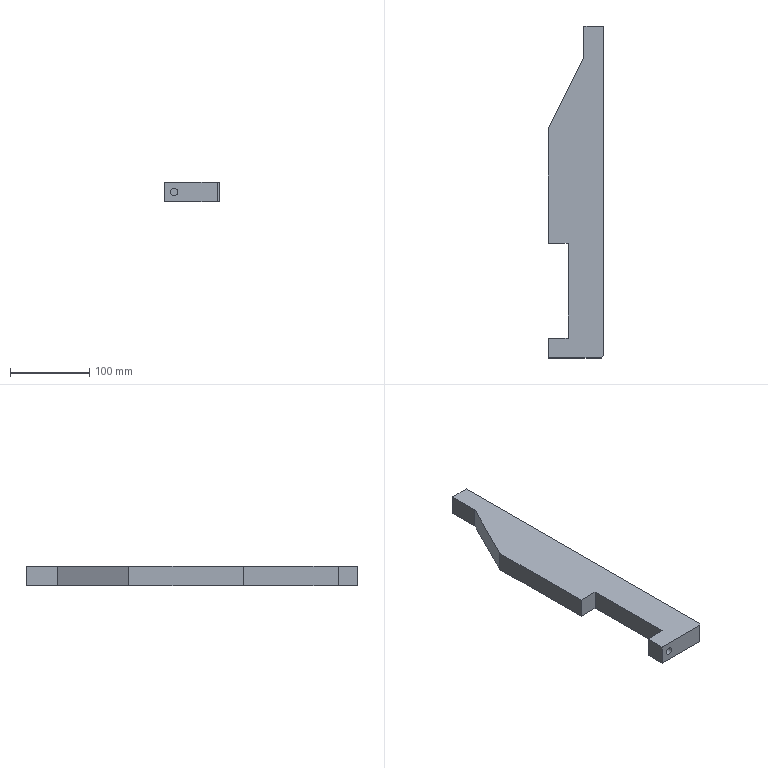Part | NX | 1 solid | 22 faces | box 70 x 420 x 25 mm | volume 559704 mm3 | plane 13 | cylinder 5 | cone 4 | commonest cylinder face diameters 6.8 x4 9 x1
STEP:
#1=CARTESIAN_POINT('',(67.,0.,12.5));
#2=VERTEX_POINT('',#1);
#3=CARTESIAN_POINT('',(70.,3.,12.5));
#4=VERTEX_POINT('',#3);
#5=CARTESIAN_POINT('',(33.5,-33.5,12.5));
#6=DIRECTION('',(0.7071,0.7071,0.));
#7=VECTOR('',#6,1000.);
#8=LINE('',#5,#7);
#9=EDGE_CURVE('',#2,#4,#8,.T.);
#10=ORIENTED_EDGE('',*,*,#9,.F.);
#11=CARTESIAN_POINT('',(67.,0.,-12.5));
#12=VERTEX_POINT('',#11);
#13=CARTESIAN_POINT('',(67.,0.,12.5));
#14=DIRECTION('',(0.,0.,1.));
#15=VECTOR('',#14,1000.);
#16=LINE('',#13,#15);
#17=EDGE_CURVE('',#12,#2,#16,.T.);
#18=ORIENTED_EDGE('',*,*,#17,.F.);
#19=CARTESIAN_POINT('',(70.,3.,-12.5));
#20=VERTEX_POINT('',#19);
#21=CARTESIAN_POINT('',(70.,3.,-12.5));
#22=DIRECTION('',(-0.7071,-0.7071,0.));
#23=VECTOR('',#22,1000.);
#24=LINE('',#21,#23);
#25=EDGE_CURVE('',#20,#12,#24,.T.);
#26=ORIENTED_EDGE('',*,*,#25,.F.);
#27=CARTESIAN_POINT('',(70.,3.,12.5));
#28=DIRECTION('',(0.,0.,-1.));
#29=VECTOR('',#28,1000.);
#30=LINE('',#27,#29);
#31=EDGE_CURVE('',#4,#20,#30,.T.);
#32=ORIENTED_EDGE('',*,*,#31,.F.);
#33=EDGE_LOOP('',(#10,#18,#26,#32));
#34=FACE_BOUND('',#33,.T.);
#35=CARTESIAN_POINT('',(70.,3.,12.5));
#36=DIRECTION('',(-0.7071,0.7071,0.));
#37=DIRECTION('',(0.,0.,-1.));
#38=AXIS2_PLACEMENT_3D('',#35,#36,#37);
#39=PLANE('',#38);
#40=ADVANCED_FACE('',(#34),#39,.F.);
#41=CARTESIAN_POINT('',(0.,290.,12.5));
#42=VERTEX_POINT('',#41);
#43=CARTESIAN_POINT('',(45.,380.,12.5));
#44=VERTEX_POINT('',#43);
#45=CARTESIAN_POINT('',(45.,380.,12.5));
#46=DIRECTION('',(0.4472,0.8944,0.));
#47=VECTOR('',#46,1000.);
#48=LINE('',#45,#47);
#49=EDGE_CURVE('',#42,#44,#48,.T.);
#50=ORIENTED_EDGE('',*,*,#49,.T.);
#51=CARTESIAN_POINT('',(45.,380.,-12.5));
#52=VERTEX_POINT('',#51);
#53=CARTESIAN_POINT('',(45.,380.,-12.5));
#54=DIRECTION('',(0.,0.,1.));
#55=VECTOR('',#54,1000.);
#56=LINE('',#53,#55);
#57=EDGE_CURVE('',#52,#44,#56,.T.);
#58=ORIENTED_EDGE('',*,*,#57,.F.);
#59=CARTESIAN_POINT('',(0.,290.,-12.5));
#60=VERTEX_POINT('',#59);
#61=CARTESIAN_POINT('',(45.,380.,-12.5));
#62=DIRECTION('',(0.4472,0.8944,0.));
#63=VECTOR('',#62,1000.);
#64=LINE('',#61,#63);
#65=EDGE_CURVE('',#60,#52,#64,.T.);
#66=ORIENTED_EDGE('',*,*,#65,.F.);
#67=CARTESIAN_POINT('',(0.,290.,-12.5));
#68=DIRECTION('',(0.,0.,1.));
#69=VECTOR('',#68,1000.);
#70=LINE('',#67,#69);
#71=EDGE_CURVE('',#60,#42,#70,.T.);
#72=ORIENTED_EDGE('',*,*,#71,.T.);
#73=EDGE_LOOP('',(#50,#58,#66,#72));
#74=FACE_BOUND('',#73,.T.);
#75=CARTESIAN_POINT('',(45.,380.,-12.5));
#76=DIRECTION('',(0.8944,-0.4472,0.));
#77=DIRECTION('',(0.4472,0.8944,0.));
#78=AXIS2_PLACEMENT_3D('',#75,#76,#77);
#79=PLANE('',#78);
#80=ADVANCED_FACE('',(#74),#79,.F.);
#81=CARTESIAN_POINT('',(45.,420.,12.5));
#82=VERTEX_POINT('',#81);
#83=CARTESIAN_POINT('',(45.,420.,12.5));
#84=DIRECTION('',(0.,1.,0.));
#85=VECTOR('',#84,1000.);
#86=LINE('',#83,#85);
#87=EDGE_CURVE('',#44,#82,#86,.T.);
#88=ORIENTED_EDGE('',*,*,#87,.T.);
#89=CARTESIAN_POINT('',(45.,420.,-12.5));
#90=VERTEX_POINT('',#89);
#91=CARTESIAN_POINT('',(45.,420.,-12.5));
#92=DIRECTION('',(0.,0.,1.));
#93=VECTOR('',#92,1000.);
#94=LINE('',#91,#93);
#95=EDGE_CURVE('',#90,#82,#94,.T.);
#96=ORIENTED_EDGE('',*,*,#95,.F.);
#97=CARTESIAN_POINT('',(45.,420.,-12.5));
#98=DIRECTION('',(0.,1.,0.));
#99=VECTOR('',#98,1000.);
#100=LINE('',#97,#99);
#101=EDGE_CURVE('',#52,#90,#100,.T.);
#102=ORIENTED_EDGE('',*,*,#101,.F.);
#103=ORIENTED_EDGE('',*,*,#57,.T.);
#104=EDGE_LOOP('',(#88,#96,#102,#103));
#105=FACE_BOUND('',#104,.T.);
#106=CARTESIAN_POINT('',(45.,420.,-12.5));
#107=DIRECTION('',(1.,0.,0.));
#108=DIRECTION('',(0.,0.,-1.));
#109=AXIS2_PLACEMENT_3D('',#106,#107,#108);
#110=PLANE('',#109);
#111=ADVANCED_FACE('',(#105),#110,.F.);
#112=CARTESIAN_POINT('',(0.,25.,12.5));
#113=VERTEX_POINT('',#112);
#114=CARTESIAN_POINT('',(25.,25.,12.5));
#115=VERTEX_POINT('',#114);
#116=CARTESIAN_POINT('',(0.,25.,12.5));
#117=DIRECTION('',(1.,0.,0.));
#118=VECTOR('',#117,1000.);
#119=LINE('',#116,#118);
#120=EDGE_CURVE('',#113,#115,#119,.T.);
#121=ORIENTED_EDGE('',*,*,#120,.T.);
#122=CARTESIAN_POINT('',(25.,25.,-12.5));
#123=VERTEX_POINT('',#122);
#124=CARTESIAN_POINT('',(25.,25.,-12.5));
#125=DIRECTION('',(0.,0.,1.));
#126=VECTOR('',#125,1000.);
#127=LINE('',#124,#126);
#128=EDGE_CURVE('',#123,#115,#127,.T.);
#129=ORIENTED_EDGE('',*,*,#128,.F.);
#130=CARTESIAN_POINT('',(0.,25.,-12.5));
#131=VERTEX_POINT('',#130);
#132=CARTESIAN_POINT('',(0.,25.,-12.5));
#133=DIRECTION('',(1.,0.,0.));
#134=VECTOR('',#133,1000.);
#135=LINE('',#132,#134);
#136=EDGE_CURVE('',#131,#123,#135,.T.);
#137=ORIENTED_EDGE('',*,*,#136,.F.);
#138=CARTESIAN_POINT('',(0.,25.,-12.5));
#139=DIRECTION('',(0.,0.,1.));
#140=VECTOR('',#139,1000.);
#141=LINE('',#138,#140);
#142=EDGE_CURVE('',#131,#113,#141,.T.);
#143=ORIENTED_EDGE('',*,*,#142,.T.);
#144=EDGE_LOOP('',(#121,#129,#137,#143));
#145=FACE_BOUND('',#144,.T.);
#146=CARTESIAN_POINT('',(12.5,25.,4.5));
#147=VERTEX_POINT('',#146);
#148=CARTESIAN_POINT('',(12.5,25.,0.));
#149=DIRECTION('',(0.,1.,0.));
#150=DIRECTION('',(0.,0.,1.));
#151=AXIS2_PLACEMENT_3D('',#148,#149,#150);
#152=CIRCLE('',#151,4.5);
#153=EDGE_CURVE('',#147,#147,#152,.T.);
#154=ORIENTED_EDGE('',*,*,#153,.F.);
#155=EDGE_LOOP('',(#154));
#156=FACE_BOUND('',#155,.T.);
#157=CARTESIAN_POINT('',(0.,25.,-12.5));
#158=DIRECTION('',(0.,-1.,0.));
#159=DIRECTION('',(1.,0.,0.));
#160=AXIS2_PLACEMENT_3D('',#157,#158,#159);
#161=PLANE('',#160);
#162=ADVANCED_FACE('',(#145,#156),#161,.F.);
#163=CARTESIAN_POINT('',(25.,145.,12.5));
#164=VERTEX_POINT('',#163);
#165=CARTESIAN_POINT('',(25.,145.,12.5));
#166=DIRECTION('',(0.,1.,0.));
#167=VECTOR('',#166,1000.);
#168=LINE('',#165,#167);
#169=EDGE_CURVE('',#115,#164,#168,.T.);
#170=ORIENTED_EDGE('',*,*,#169,.T.);
#171=CARTESIAN_POINT('',(25.,145.,-12.5));
#172=VERTEX_POINT('',#171);
#173=CARTESIAN_POINT('',(25.,145.,-12.5));
#174=DIRECTION('',(0.,0.,1.));
#175=VECTOR('',#174,1000.);
#176=LINE('',#173,#175);
#177=EDGE_CURVE('',#172,#164,#176,.T.);
#178=ORIENTED_EDGE('',*,*,#177,.F.);
#179=CARTESIAN_POINT('',(25.,145.,-12.5));
#180=DIRECTION('',(0.,1.,0.));
#181=VECTOR('',#180,1000.);
#182=LINE('',#179,#181);
#183=EDGE_CURVE('',#123,#172,#182,.T.);
#184=ORIENTED_EDGE('',*,*,#183,.F.);
#185=ORIENTED_EDGE('',*,*,#128,.T.);
#186=EDGE_LOOP('',(#170,#178,#184,#185));
#187=FACE_BOUND('',#186,.T.);
#188=CARTESIAN_POINT('',(25.,145.,-12.5));
#189=DIRECTION('',(1.,0.,0.));
#190=DIRECTION('',(0.,1.,0.));
#191=AXIS2_PLACEMENT_3D('',#188,#189,#190);
#192=PLANE('',#191);
#193=ADVANCED_FACE('',(#187),#192,.F.);
#194=CARTESIAN_POINT('',(0.,145.,12.5));
#195=VERTEX_POINT('',#194);
#196=CARTESIAN_POINT('',(0.,145.,12.5));
#197=DIRECTION('',(-1.,0.,0.));
#198=VECTOR('',#197,1000.);
#199=LINE('',#196,#198);
#200=EDGE_CURVE('',#164,#195,#199,.T.);
#201=ORIENTED_EDGE('',*,*,#200,.T.);
#202=CARTESIAN_POINT('',(0.,145.,-12.5));
#203=VERTEX_POINT('',#202);
#204=CARTESIAN_POINT('',(0.,145.,-12.5));
#205=DIRECTION('',(0.,0.,1.));
#206=VECTOR('',#205,1000.);
#207=LINE('',#204,#206);
#208=EDGE_CURVE('',#203,#195,#207,.T.);
#209=ORIENTED_EDGE('',*,*,#208,.F.);
#210=CARTESIAN_POINT('',(0.,145.,-12.5));
#211=DIRECTION('',(-1.,0.,0.));
#212=VECTOR('',#211,1000.);
#213=LINE('',#210,#212);
#214=EDGE_CURVE('',#172,#203,#213,.T.);
#215=ORIENTED_EDGE('',*,*,#214,.F.);
#216=ORIENTED_EDGE('',*,*,#177,.T.);
#217=EDGE_LOOP('',(#201,#209,#215,#216));
#218=FACE_BOUND('',#217,.T.);
#219=CARTESIAN_POINT('',(0.,145.,-12.5));
#220=DIRECTION('',(0.,1.,0.));
#221=DIRECTION('',(0.,0.,1.));
#222=AXIS2_PLACEMENT_3D('',#219,#220,#221);
#223=PLANE('',#222);
#224=ADVANCED_FACE('',(#218),#223,.F.);
#225=CARTESIAN_POINT('',(70.,420.,-12.5));
#226=VERTEX_POINT('',#225);
#227=CARTESIAN_POINT('',(70.,0.,-12.5));
#228=DIRECTION('',(0.,1.,0.));
#229=VECTOR('',#228,1000.);
#230=LINE('',#227,#229);
#231=EDGE_CURVE('',#20,#226,#230,.T.);
#232=ORIENTED_EDGE('',*,*,#231,.F.);
#233=ORIENTED_EDGE('',*,*,#25,.T.);
#234=CARTESIAN_POINT('',(0.,0.,-12.5));
#235=VERTEX_POINT('',#234);
#236=CARTESIAN_POINT('',(0.,0.,-12.5));
#237=DIRECTION('',(1.,0.,0.));
#238=VECTOR('',#237,1000.);
#239=LINE('',#236,#238);
#240=EDGE_CURVE('',#235,#12,#239,.T.);
#241=ORIENTED_EDGE('',*,*,#240,.F.);
#242=CARTESIAN_POINT('',(0.,420.,-12.5));
#243=DIRECTION('',(0.,-1.,0.));
#244=VECTOR('',#243,1000.);
#245=LINE('',#242,#244);
#246=EDGE_CURVE('',#131,#235,#245,.T.);
#247=ORIENTED_EDGE('',*,*,#246,.F.);
#248=ORIENTED_EDGE('',*,*,#136,.T.);
#249=ORIENTED_EDGE('',*,*,#183,.T.);
#250=ORIENTED_EDGE('',*,*,#214,.T.);
#251=CARTESIAN_POINT('',(0.,420.,-12.5));
#252=DIRECTION('',(0.,-1.,0.));
#253=VECTOR('',#252,1000.);
#254=LINE('',#251,#253);
#255=EDGE_CURVE('',#60,#203,#254,.T.);
#256=ORIENTED_EDGE('',*,*,#255,.F.);
#257=ORIENTED_EDGE('',*,*,#65,.T.);
#258=ORIENTED_EDGE('',*,*,#101,.T.);
#259=CARTESIAN_POINT('',(70.,420.,-12.5));
#260=DIRECTION('',(-1.,0.,0.));
#261=VECTOR('',#260,1000.);
#262=LINE('',#259,#261);
#263=EDGE_CURVE('',#226,#90,#262,.T.);
#264=ORIENTED_EDGE('',*,*,#263,.F.);
#265=EDGE_LOOP('',(#232,#233,#241,#247,#248,#249,#250,#256,#257,#258,#264));
#266=FACE_BOUND('',#265,.T.);
#267=CARTESIAN_POINT('',(0.,0.,-12.5));
#268=DIRECTION('',(0.,0.,1.));
#269=DIRECTION('',(1.,0.,0.));
#270=AXIS2_PLACEMENT_3D('',#267,#268,#269);
#271=PLANE('',#270);
#272=ADVANCED_FACE('',(#266),#271,.F.);
#273=CARTESIAN_POINT('',(0.,0.,12.5));
#274=VERTEX_POINT('',#273);
#275=CARTESIAN_POINT('',(0.,0.,12.5));
#276=DIRECTION('',(1.,0.,0.));
#277=VECTOR('',#276,1000.);
#278=LINE('',#275,#277);
#279=EDGE_CURVE('',#274,#2,#278,.T.);
#280=ORIENTED_EDGE('',*,*,#279,.T.);
#281=ORIENTED_EDGE('',*,*,#9,.T.);
#282=CARTESIAN_POINT('',(70.,420.,12.5));
#283=VERTEX_POINT('',#282);
#284=CARTESIAN_POINT('',(70.,0.,12.5));
#285=DIRECTION('',(0.,1.,0.));
#286=VECTOR('',#285,1000.);
#287=LINE('',#284,#286);
#288=EDGE_CURVE('',#4,#283,#287,.T.);
#289=ORIENTED_EDGE('',*,*,#288,.T.);
#290=CARTESIAN_POINT('',(70.,420.,12.5));
#291=DIRECTION('',(-1.,0.,0.));
#292=VECTOR('',#291,1000.);
#293=LINE('',#290,#292);
#294=EDGE_CURVE('',#283,#82,#293,.T.);
#295=ORIENTED_EDGE('',*,*,#294,.T.);
#296=ORIENTED_EDGE('',*,*,#87,.F.);
#297=ORIENTED_EDGE('',*,*,#49,.F.);
#298=CARTESIAN_POINT('',(0.,420.,12.5));
#299=DIRECTION('',(0.,-1.,0.));
#300=VECTOR('',#299,1000.);
#301=LINE('',#298,#300);
#302=EDGE_CURVE('',#42,#195,#301,.T.);
#303=ORIENTED_EDGE('',*,*,#302,.T.);
#304=ORIENTED_EDGE('',*,*,#200,.F.);
#305=ORIENTED_EDGE('',*,*,#169,.F.);
#306=ORIENTED_EDGE('',*,*,#120,.F.);
#307=CARTESIAN_POINT('',(0.,420.,12.5));
#308=DIRECTION('',(0.,-1.,0.));
#309=VECTOR('',#308,1000.);
#310=LINE('',#307,#309);
#311=EDGE_CURVE('',#113,#274,#310,.T.);
#312=ORIENTED_EDGE('',*,*,#311,.T.);
#313=EDGE_LOOP('',(#280,#281,#289,#295,#296,#297,#303,#304,#305,#306,#312));
#314=FACE_BOUND('',#313,.T.);
#315=CARTESIAN_POINT('',(0.,0.,12.5));
#316=DIRECTION('',(0.,0.,1.));
#317=DIRECTION('',(1.,0.,0.));
#318=AXIS2_PLACEMENT_3D('',#315,#316,#317);
#319=PLANE('',#318);
#320=ADVANCED_FACE('',(#314),#319,.T.);
#321=ORIENTED_EDGE('',*,*,#263,.T.);
#322=ORIENTED_EDGE('',*,*,#95,.T.);
#323=ORIENTED_EDGE('',*,*,#294,.F.);
#324=CARTESIAN_POINT('',(70.,420.,12.5));
#325=DIRECTION('',(0.,0.,-1.));
#326=VECTOR('',#325,1000.);
#327=LINE('',#324,#326);
#328=EDGE_CURVE('',#283,#226,#327,.T.);
#329=ORIENTED_EDGE('',*,*,#328,.T.);
#330=EDGE_LOOP('',(#321,#322,#323,#329));
#331=FACE_BOUND('',#330,.T.);
#332=CARTESIAN_POINT('',(70.,420.,12.5));
#333=DIRECTION('',(0.,-1.,0.));
#334=DIRECTION('',(0.,0.,-1.));
#335=AXIS2_PLACEMENT_3D('',#332,#333,#334);
#336=PLANE('',#335);
#337=ADVANCED_FACE('',(#331),#336,.F.);
#338=ORIENTED_EDGE('',*,*,#288,.F.);
#339=ORIENTED_EDGE('',*,*,#31,.T.);
#340=ORIENTED_EDGE('',*,*,#231,.T.);
#341=ORIENTED_EDGE('',*,*,#328,.F.);
#342=EDGE_LOOP('',(#338,#339,#340,#341));
#343=FACE_BOUND('',#342,.T.);
#344=CARTESIAN_POINT('',(70.,410.,-3.4));
#345=VERTEX_POINT('',#344);
#346=CARTESIAN_POINT('',(70.,410.,0.));
#347=DIRECTION('',(1.,0.,0.));
#348=DIRECTION('',(0.,0.,-1.));
#349=AXIS2_PLACEMENT_3D('',#346,#347,#348);
#350=CIRCLE('',#349,3.4);
#351=EDGE_CURVE('',#345,#345,#350,.T.);
#352=ORIENTED_EDGE('',*,*,#351,.F.);
#353=EDGE_LOOP('',(#352));
#354=FACE_BOUND('',#353,.T.);
#355=CARTESIAN_POINT('',(70.,290.,-3.4));
#356=VERTEX_POINT('',#355);
#357=CARTESIAN_POINT('',(70.,290.,0.));
#358=DIRECTION('',(1.,0.,0.));
#359=DIRECTION('',(0.,0.,-1.));
#360=AXIS2_PLACEMENT_3D('',#357,#358,#359);
#361=CIRCLE('',#360,3.4);
#362=EDGE_CURVE('',#356,#356,#361,.T.);
#363=ORIENTED_EDGE('',*,*,#362,.F.);
#364=EDGE_LOOP('',(#363));
#365=FACE_BOUND('',#364,.T.);
#366=CARTESIAN_POINT('',(70.,170.,-3.4));
#367=VERTEX_POINT('',#366);
#368=CARTESIAN_POINT('',(70.,170.,0.));
#369=DIRECTION('',(1.,0.,0.));
#370=DIRECTION('',(0.,0.,-1.));
#371=AXIS2_PLACEMENT_3D('',#368,#369,#370);
#372=CIRCLE('',#371,3.4);
#373=EDGE_CURVE('',#367,#367,#372,.T.);
#374=ORIENTED_EDGE('',*,*,#373,.F.);
#375=EDGE_LOOP('',(#374));
#376=FACE_BOUND('',#375,.T.);
#377=CARTESIAN_POINT('',(70.,50.,-3.4));
#378=VERTEX_POINT('',#377);
#379=CARTESIAN_POINT('',(70.,50.,0.));
#380=DIRECTION('',(1.,0.,0.));
#381=DIRECTION('',(0.,0.,-1.));
#382=AXIS2_PLACEMENT_3D('',#379,#380,#381);
#383=CIRCLE('',#382,3.4);
#384=EDGE_CURVE('',#378,#378,#383,.T.);
#385=ORIENTED_EDGE('',*,*,#384,.F.);
#386=EDGE_LOOP('',(#385));
#387=FACE_BOUND('',#386,.T.);
#388=CARTESIAN_POINT('',(70.,0.,12.5));
#389=DIRECTION('',(-1.,0.,0.));
#390=DIRECTION('',(0.,0.,1.));
#391=AXIS2_PLACEMENT_3D('',#388,#389,#390);
#392=PLANE('',#391);
#393=ADVANCED_FACE('',(#343,#354,#365,#376,#387),#392,.F.);
#394=ORIENTED_EDGE('',*,*,#240,.T.);
#395=ORIENTED_EDGE('',*,*,#17,.T.);
#396=ORIENTED_EDGE('',*,*,#279,.F.);
#397=CARTESIAN_POINT('',(0.,0.,12.5));
#398=DIRECTION('',(0.,0.,-1.));
#399=VECTOR('',#398,1000.);
#400=LINE('',#397,#399);
#401=EDGE_CURVE('',#274,#235,#400,.T.);
#402=ORIENTED_EDGE('',*,*,#401,.T.);
#403=EDGE_LOOP('',(#394,#395,#396,#402));
#404=FACE_BOUND('',#403,.T.);
#405=CARTESIAN_POINT('',(12.5,0.,4.5));
#406=VERTEX_POINT('',#405);
#407=CARTESIAN_POINT('',(12.5,0.,0.));
#408=DIRECTION('',(0.,1.,0.));
#409=DIRECTION('',(0.,0.,1.));
#410=AXIS2_PLACEMENT_3D('',#407,#408,#409);
#411=CIRCLE('',#410,4.5);
#412=EDGE_CURVE('',#406,#406,#411,.T.);
#413=ORIENTED_EDGE('',*,*,#412,.T.);
#414=EDGE_LOOP('',(#413));
#415=FACE_BOUND('',#414,.T.);
#416=CARTESIAN_POINT('',(0.,0.,12.5));
#417=DIRECTION('',(0.,1.,0.));
#418=DIRECTION('',(0.,0.,1.));
#419=AXIS2_PLACEMENT_3D('',#416,#417,#418);
#420=PLANE('',#419);
#421=ADVANCED_FACE('',(#404,#415),#420,.F.);
#422=ORIENTED_EDGE('',*,*,#311,.F.);
#423=ORIENTED_EDGE('',*,*,#142,.F.);
#424=ORIENTED_EDGE('',*,*,#246,.T.);
#425=ORIENTED_EDGE('',*,*,#401,.F.);
#426=EDGE_LOOP('',(#422,#423,#424,#425));
#427=FACE_BOUND('',#426,.T.);
#428=CARTESIAN_POINT('',(0.,420.,12.5));
#429=DIRECTION('',(1.,0.,0.));
#430=DIRECTION('',(0.,1.,0.));
#431=AXIS2_PLACEMENT_3D('',#428,#429,#430);
#432=PLANE('',#431);
#433=ADVANCED_FACE('',(#427),#432,.F.);
#434=ORIENTED_EDGE('',*,*,#302,.F.);
#435=ORIENTED_EDGE('',*,*,#71,.F.);
#436=ORIENTED_EDGE('',*,*,#255,.T.);
#437=ORIENTED_EDGE('',*,*,#208,.T.);
#438=EDGE_LOOP('',(#434,#435,#436,#437));
#439=FACE_BOUND('',#438,.T.);
#440=CARTESIAN_POINT('',(0.,420.,12.5));
#441=DIRECTION('',(1.,0.,0.));
#442=DIRECTION('',(0.,1.,0.));
#443=AXIS2_PLACEMENT_3D('',#440,#441,#442);
#444=PLANE('',#443);
#445=ADVANCED_FACE('',(#439),#444,.F.);
#446=CARTESIAN_POINT('',(48.207,410.,0.));
#447=VERTEX_POINT('',#446);
#448=VERTEX_LOOP('',#447);
#449=FACE_BOUND('',#448,.T.);
#450=CARTESIAN_POINT('',(50.25,410.,-3.4));
#451=VERTEX_POINT('',#450);
#452=CARTESIAN_POINT('',(50.25,410.,0.));
#453=DIRECTION('',(1.,0.,0.));
#454=DIRECTION('',(0.,0.,-1.));
#455=AXIS2_PLACEMENT_3D('',#452,#453,#454);
#456=CIRCLE('',#455,3.4);
#457=EDGE_CURVE('',#451,#451,#456,.T.);
#458=ORIENTED_EDGE('',*,*,#457,.T.);
#459=EDGE_LOOP('',(#458));
#460=FACE_BOUND('',#459,.T.);
#461=CARTESIAN_POINT('',(50.25,410.,0.));
#462=DIRECTION('',(1.,0.,0.));
#463=DIRECTION('',(0.,0.,-1.));
#464=AXIS2_PLACEMENT_3D('',#461,#462,#463);
#465=CONICAL_SURFACE('',#464,3.4,1.03);
#466=ADVANCED_FACE('',(#449,#460),#465,.F.);
#467=ORIENTED_EDGE('',*,*,#351,.T.);
#468=EDGE_LOOP('',(#467));
#469=FACE_BOUND('',#468,.T.);
#470=ORIENTED_EDGE('',*,*,#457,.F.);
#471=EDGE_LOOP('',(#470));
#472=FACE_BOUND('',#471,.T.);
#473=CARTESIAN_POINT('',(70.,410.,0.));
#474=DIRECTION('',(1.,0.,0.));
#475=DIRECTION('',(0.,0.,-1.));
#476=AXIS2_PLACEMENT_3D('',#473,#474,#475);
#477=CYLINDRICAL_SURFACE('',#476,3.4);
#478=ADVANCED_FACE('',(#469,#472),#477,.F.);
#479=CARTESIAN_POINT('',(48.207,290.,0.));
#480=VERTEX_POINT('',#479);
#481=VERTEX_LOOP('',#480);
#482=FACE_BOUND('',#481,.T.);
#483=CARTESIAN_POINT('',(50.25,290.,-3.4));
#484=VERTEX_POINT('',#483);
#485=CARTESIAN_POINT('',(50.25,290.,0.));
#486=DIRECTION('',(1.,0.,0.));
#487=DIRECTION('',(0.,0.,-1.));
#488=AXIS2_PLACEMENT_3D('',#485,#486,#487);
#489=CIRCLE('',#488,3.4);
#490=EDGE_CURVE('',#484,#484,#489,.T.);
#491=ORIENTED_EDGE('',*,*,#490,.T.);
#492=EDGE_LOOP('',(#491));
#493=FACE_BOUND('',#492,.T.);
#494=CARTESIAN_POINT('',(50.25,290.,0.));
#495=DIRECTION('',(1.,0.,0.));
#496=DIRECTION('',(0.,0.,-1.));
#497=AXIS2_PLACEMENT_3D('',#494,#495,#496);
#498=CONICAL_SURFACE('',#497,3.4,1.03);
#499=ADVANCED_FACE('',(#482,#493),#498,.F.);
#500=ORIENTED_EDGE('',*,*,#362,.T.);
#501=EDGE_LOOP('',(#500));
#502=FACE_BOUND('',#501,.T.);
#503=ORIENTED_EDGE('',*,*,#490,.F.);
#504=EDGE_LOOP('',(#503));
#505=FACE_BOUND('',#504,.T.);
#506=CARTESIAN_POINT('',(70.,290.,0.));
#507=DIRECTION('',(1.,0.,0.));
#508=DIRECTION('',(0.,0.,-1.));
#509=AXIS2_PLACEMENT_3D('',#506,#507,#508);
#510=CYLINDRICAL_SURFACE('',#509,3.4);
#511=ADVANCED_FACE('',(#502,#505),#510,.F.);
#512=CARTESIAN_POINT('',(48.207,170.,0.));
#513=VERTEX_POINT('',#512);
#514=VERTEX_LOOP('',#513);
#515=FACE_BOUND('',#514,.T.);
#516=CARTESIAN_POINT('',(50.25,170.,-3.4));
#517=VERTEX_POINT('',#516);
#518=CARTESIAN_POINT('',(50.25,170.,0.));
#519=DIRECTION('',(1.,0.,0.));
#520=DIRECTION('',(0.,0.,-1.));
#521=AXIS2_PLACEMENT_3D('',#518,#519,#520);
#522=CIRCLE('',#521,3.4);
#523=EDGE_CURVE('',#517,#517,#522,.T.);
#524=ORIENTED_EDGE('',*,*,#523,.T.);
#525=EDGE_LOOP('',(#524));
#526=FACE_BOUND('',#525,.T.);
#527=CARTESIAN_POINT('',(50.25,170.,0.));
#528=DIRECTION('',(1.,0.,0.));
#529=DIRECTION('',(0.,0.,-1.));
#530=AXIS2_PLACEMENT_3D('',#527,#528,#529);
#531=CONICAL_SURFACE('',#530,3.4,1.03);
#532=ADVANCED_FACE('',(#515,#526),#531,.F.);
#533=ORIENTED_EDGE('',*,*,#373,.T.);
#534=EDGE_LOOP('',(#533));
#535=FACE_BOUND('',#534,.T.);
#536=ORIENTED_EDGE('',*,*,#523,.F.);
#537=EDGE_LOOP('',(#536));
#538=FACE_BOUND('',#537,.T.);
#539=CARTESIAN_POINT('',(70.,170.,0.));
#540=DIRECTION('',(1.,0.,0.));
#541=DIRECTION('',(0.,0.,-1.));
#542=AXIS2_PLACEMENT_3D('',#539,#540,#541);
#543=CYLINDRICAL_SURFACE('',#542,3.4);
#544=ADVANCED_FACE('',(#535,#538),#543,.F.);
#545=CARTESIAN_POINT('',(48.207,50.,0.));
#546=VERTEX_POINT('',#545);
#547=VERTEX_LOOP('',#546);
#548=FACE_BOUND('',#547,.T.);
#549=CARTESIAN_POINT('',(50.25,50.,-3.4));
#550=VERTEX_POINT('',#549);
#551=CARTESIAN_POINT('',(50.25,50.,0.));
#552=DIRECTION('',(1.,0.,0.));
#553=DIRECTION('',(0.,0.,-1.));
#554=AXIS2_PLACEMENT_3D('',#551,#552,#553);
#555=CIRCLE('',#554,3.4);
#556=EDGE_CURVE('',#550,#550,#555,.T.);
#557=ORIENTED_EDGE('',*,*,#556,.T.);
#558=EDGE_LOOP('',(#557));
#559=FACE_BOUND('',#558,.T.);
#560=CARTESIAN_POINT('',(50.25,50.,0.));
#561=DIRECTION('',(1.,0.,0.));
#562=DIRECTION('',(0.,0.,-1.));
#563=AXIS2_PLACEMENT_3D('',#560,#561,#562);
#564=CONICAL_SURFACE('',#563,3.4,1.03);
#565=ADVANCED_FACE('',(#548,#559),#564,.F.);
#566=ORIENTED_EDGE('',*,*,#384,.T.);
#567=EDGE_LOOP('',(#566));
#568=FACE_BOUND('',#567,.T.);
#569=ORIENTED_EDGE('',*,*,#556,.F.);
#570=EDGE_LOOP('',(#569));
#571=FACE_BOUND('',#570,.T.);
#572=CARTESIAN_POINT('',(70.,50.,0.));
#573=DIRECTION('',(1.,0.,0.));
#574=DIRECTION('',(0.,0.,-1.));
#575=AXIS2_PLACEMENT_3D('',#572,#573,#574);
#576=CYLINDRICAL_SURFACE('',#575,3.4);
#577=ADVANCED_FACE('',(#568,#571),#576,.F.);
#578=ORIENTED_EDGE('',*,*,#412,.F.);
#579=EDGE_LOOP('',(#578));
#580=FACE_BOUND('',#579,.T.);
#581=ORIENTED_EDGE('',*,*,#153,.T.);
#582=EDGE_LOOP('',(#581));
#583=FACE_BOUND('',#582,.T.);
#584=CARTESIAN_POINT('',(12.5,25.,0.));
#585=DIRECTION('',(0.,1.,0.));
#586=DIRECTION('',(0.,0.,1.));
#587=AXIS2_PLACEMENT_3D('',#584,#585,#586);
#588=CYLINDRICAL_SURFACE('',#587,4.5);
#589=ADVANCED_FACE('',(#580,#583),#588,.F.);
#590=CLOSED_SHELL('',(#40,#80,#111,#162,#193,#224,#272,#320,#337,#393,#421,#433,#445,#466,#478,#499,#511,#532,#544,#565,#577,#589));
#591=MANIFOLD_SOLID_BREP('',#590);
#592=(LENGTH_UNIT()NAMED_UNIT(*)SI_UNIT(.MILLI.,.METRE.));
#593=UNCERTAINTY_MEASURE_WITH_UNIT(LENGTH_MEASURE(0.00001),#592,'','');
#594=(NAMED_UNIT(*)PLANE_ANGLE_UNIT()SI_UNIT($,.RADIAN.));
#595=(NAMED_UNIT(*)SI_UNIT($,.STERADIAN.)SOLID_ANGLE_UNIT());
#596=(GEOMETRIC_REPRESENTATION_CONTEXT(3)GLOBAL_UNCERTAINTY_ASSIGNED_CONTEXT((#593))GLOBAL_UNIT_ASSIGNED_CONTEXT((#592,#594,#595))REPRESENTATION_CONTEXT('',''));
#597=ADVANCED_BREP_SHAPE_REPRESENTATION('',(#591),#596);